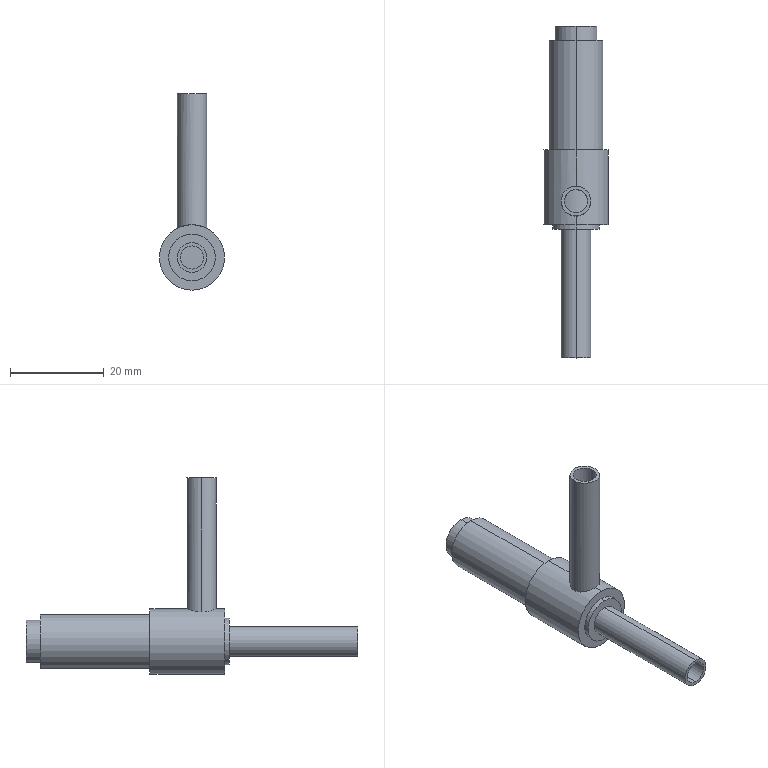Part | STEP file | 1-4 solenoid valve | 1 solid | 29 faces | box 14 x 71 x 42 mm | volume 5783 mm3 | cylinder 19 | plane 8 | cone 2 | commonest cylinder face diameters 4.95 x4 6.35 x4 14 x3 3.3 x2 9 x2 10 x2